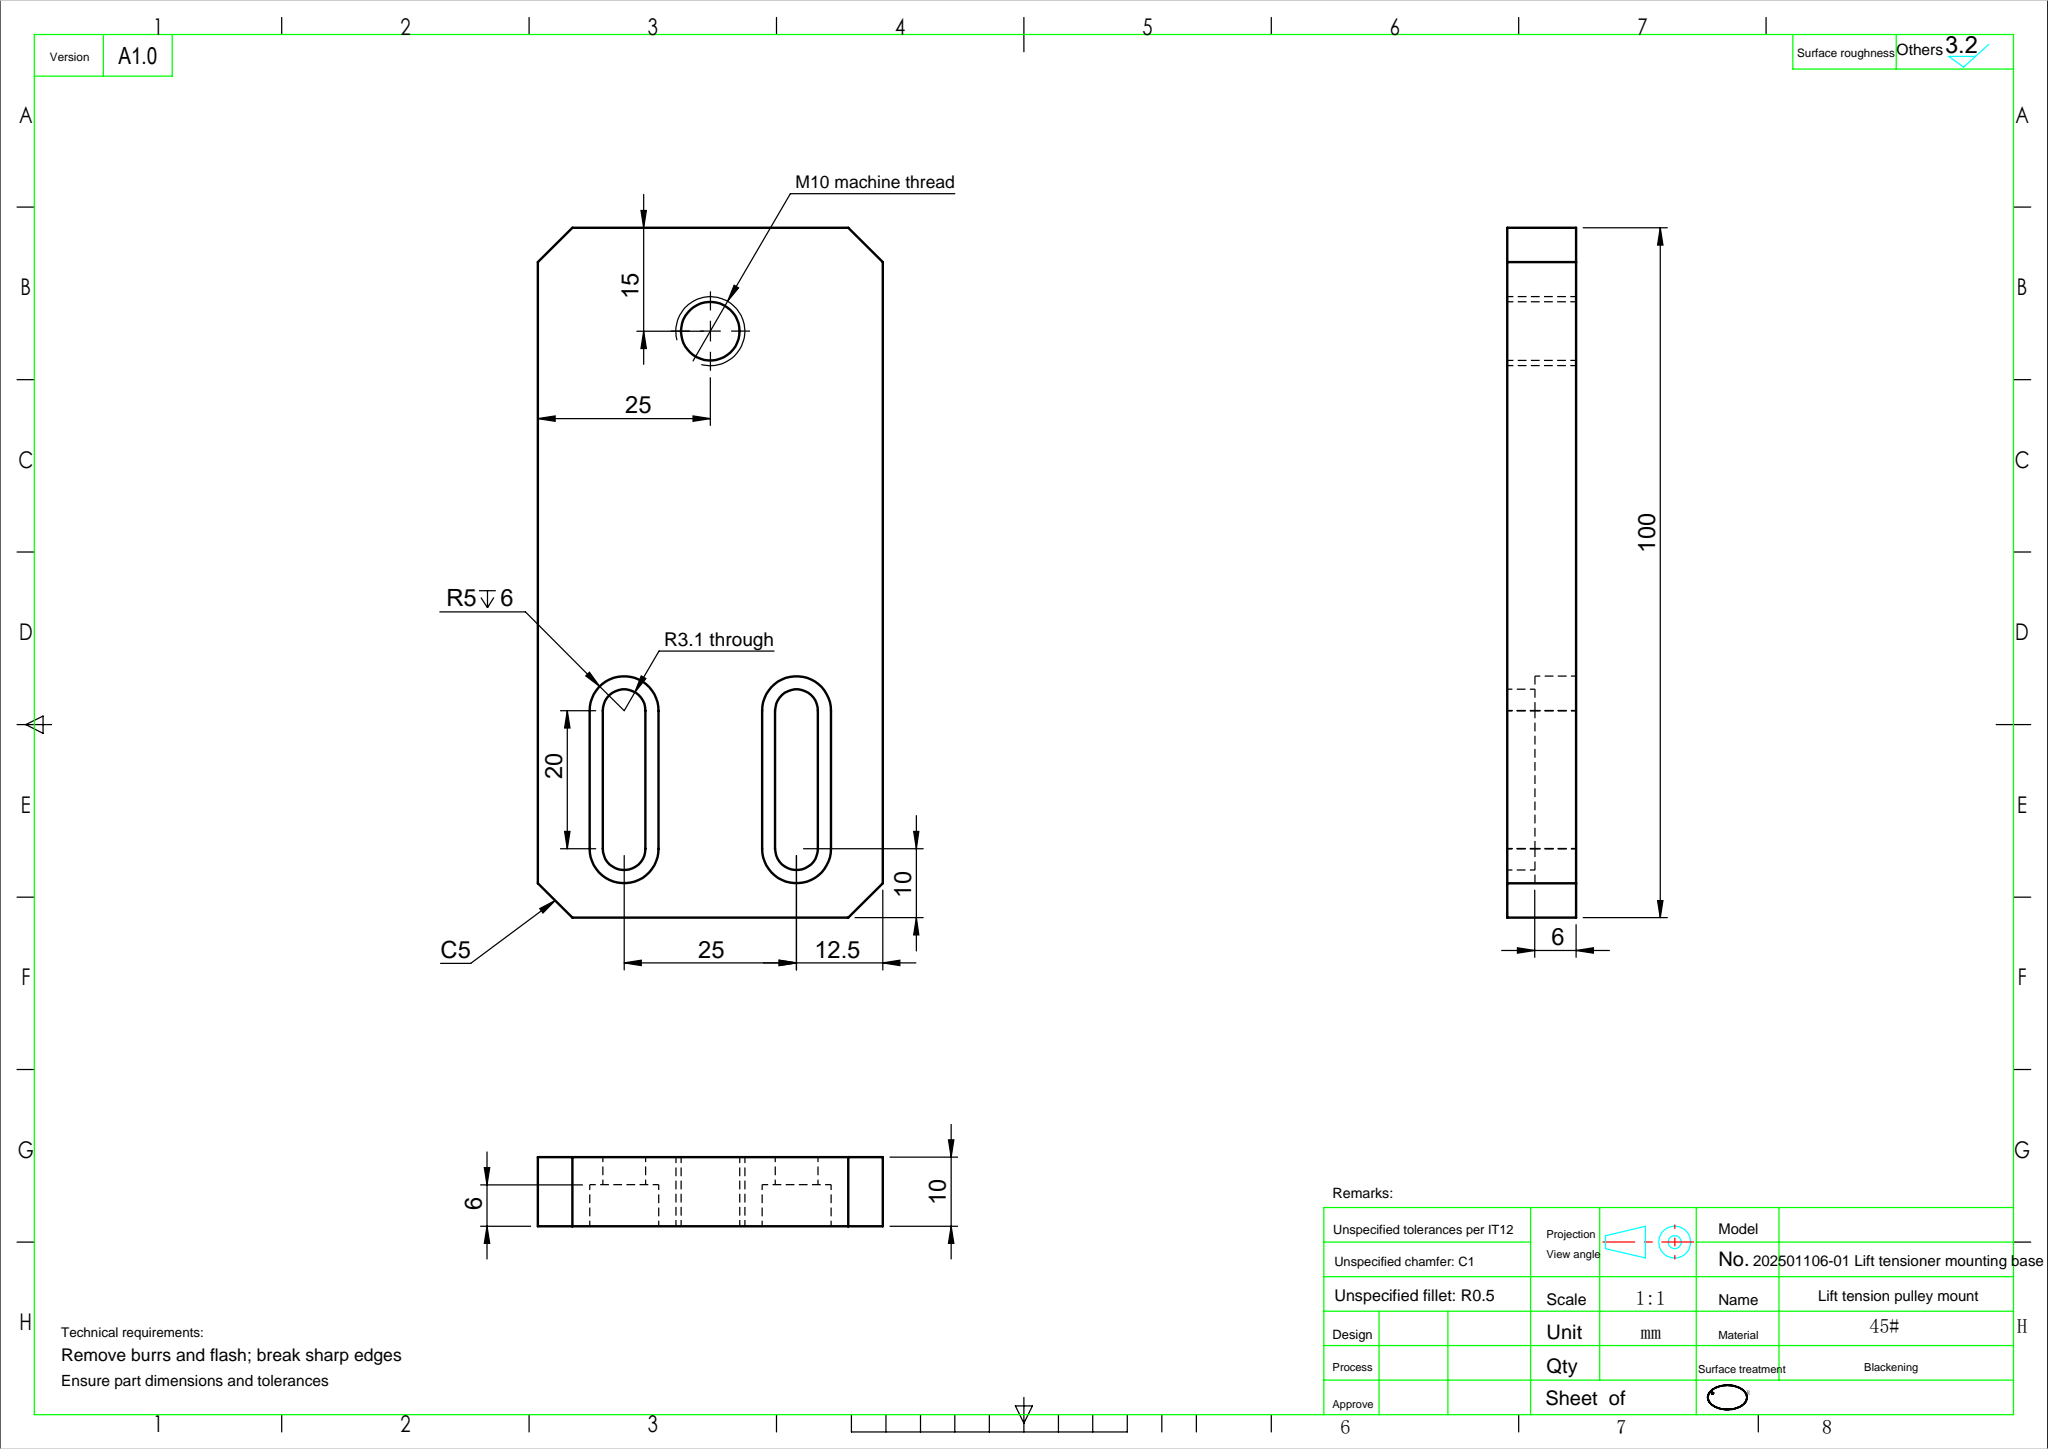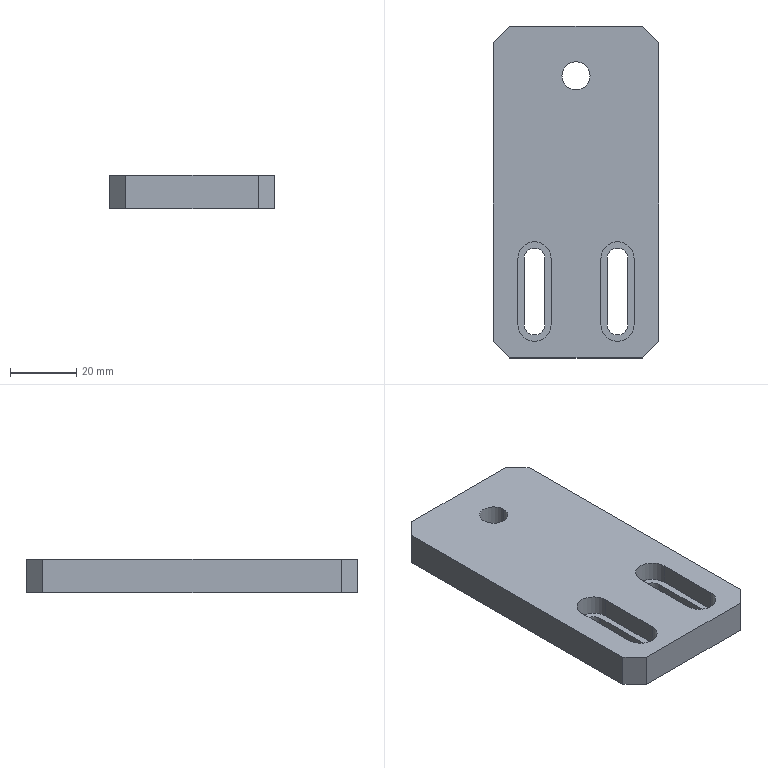Part | SolidWorks | features ICE 3, Chamfer 1, Extrusion 1 | 1 solid | 30 faces | box 50 x 100 x 10 mm | volume 44357 mm3 | plane 20 | cylinder 10 | commonest cylinder face diameters 6.2 x4 10 x4 8.5 x2
STEP:
#1=CARTESIAN_POINT('',(-4.25,35.,0.));
#2=VERTEX_POINT('',#1);
#3=CARTESIAN_POINT('',(4.25,35.,0.));
#4=VERTEX_POINT('',#3);
#5=CARTESIAN_POINT('',(0.,35.,0.));
#6=DIRECTION('',(0.,0.,1.));
#7=DIRECTION('',(1.,0.,0.));
#8=AXIS2_PLACEMENT_3D('',#5,#6,#7);
#9=CIRCLE('',#8,4.25);
#10=EDGE_CURVE('',#2,#4,#9,.T.);
#11=ORIENTED_EDGE('',*,*,#10,.F.);
#12=CARTESIAN_POINT('',(-4.25,35.,10.));
#13=VERTEX_POINT('',#12);
#14=CARTESIAN_POINT('',(-4.25,35.,0.));
#15=DIRECTION('',(0.,0.,1.));
#16=VECTOR('',#15,1000.);
#17=LINE('',#14,#16);
#18=EDGE_CURVE('',#2,#13,#17,.T.);
#19=ORIENTED_EDGE('',*,*,#18,.T.);
#20=CARTESIAN_POINT('',(4.25,35.,10.));
#21=VERTEX_POINT('',#20);
#22=CARTESIAN_POINT('',(0.,35.,10.));
#23=DIRECTION('',(0.,0.,1.));
#24=DIRECTION('',(1.,0.,0.));
#25=AXIS2_PLACEMENT_3D('',#22,#23,#24);
#26=CIRCLE('',#25,4.25);
#27=EDGE_CURVE('',#13,#21,#26,.T.);
#28=ORIENTED_EDGE('',*,*,#27,.T.);
#29=CARTESIAN_POINT('',(4.25,35.,0.));
#30=DIRECTION('',(0.,0.,1.));
#31=VECTOR('',#30,1000.);
#32=LINE('',#29,#31);
#33=EDGE_CURVE('',#4,#21,#32,.T.);
#34=ORIENTED_EDGE('',*,*,#33,.F.);
#35=EDGE_LOOP('',(#11,#19,#28,#34));
#36=FACE_OUTER_BOUND('',#35,.T.);
#37=CARTESIAN_POINT('',(0.,35.,0.));
#38=DIRECTION('',(0.,0.,1.));
#39=DIRECTION('',(1.,0.,0.));
#40=AXIS2_PLACEMENT_3D('',#37,#38,#39);
#41=CYLINDRICAL_SURFACE('',#40,4.25);
#42=ADVANCED_FACE('',(#36),#41,.F.);
#43=CARTESIAN_POINT('',(15.6,-40.,4.));
#44=VERTEX_POINT('',#43);
#45=CARTESIAN_POINT('',(9.4,-40.,4.));
#46=VERTEX_POINT('',#45);
#47=CARTESIAN_POINT('',(12.5,-40.,4.));
#48=DIRECTION('',(0.,0.,-1.));
#49=DIRECTION('',(1.,0.,0.));
#50=AXIS2_PLACEMENT_3D('',#47,#48,#49);
#51=CIRCLE('',#50,3.1);
#52=EDGE_CURVE('',#44,#46,#51,.T.);
#53=ORIENTED_EDGE('',*,*,#52,.F.);
#54=CARTESIAN_POINT('',(15.6,-40.,0.));
#55=VERTEX_POINT('',#54);
#56=CARTESIAN_POINT('',(15.6,-40.,0.));
#57=DIRECTION('',(0.,0.,1.));
#58=VECTOR('',#57,1000.);
#59=LINE('',#56,#58);
#60=EDGE_CURVE('',#55,#44,#59,.T.);
#61=ORIENTED_EDGE('',*,*,#60,.F.);
#62=CARTESIAN_POINT('',(9.4,-40.,0.));
#63=VERTEX_POINT('',#62);
#64=CARTESIAN_POINT('',(12.5,-40.,0.));
#65=DIRECTION('',(0.,0.,1.));
#66=DIRECTION('',(1.,0.,0.));
#67=AXIS2_PLACEMENT_3D('',#64,#65,#66);
#68=CIRCLE('',#67,3.1);
#69=EDGE_CURVE('',#63,#55,#68,.T.);
#70=ORIENTED_EDGE('',*,*,#69,.F.);
#71=CARTESIAN_POINT('',(9.4,-40.,0.));
#72=DIRECTION('',(0.,0.,1.));
#73=VECTOR('',#72,1000.);
#74=LINE('',#71,#73);
#75=EDGE_CURVE('',#63,#46,#74,.T.);
#76=ORIENTED_EDGE('',*,*,#75,.T.);
#77=EDGE_LOOP('',(#53,#61,#70,#76));
#78=FACE_OUTER_BOUND('',#77,.T.);
#79=CARTESIAN_POINT('',(12.5,-40.,0.));
#80=DIRECTION('',(0.,0.,1.));
#81=DIRECTION('',(1.,0.,0.));
#82=AXIS2_PLACEMENT_3D('',#79,#80,#81);
#83=CYLINDRICAL_SURFACE('',#82,3.1);
#84=ADVANCED_FACE('',(#78),#83,.F.);
#85=CARTESIAN_POINT('',(9.4,-20.,4.));
#86=VERTEX_POINT('',#85);
#87=CARTESIAN_POINT('',(9.4,-40.,4.));
#88=DIRECTION('',(0.,1.,0.));
#89=VECTOR('',#88,1000.);
#90=LINE('',#87,#89);
#91=EDGE_CURVE('',#46,#86,#90,.T.);
#92=ORIENTED_EDGE('',*,*,#91,.F.);
#93=ORIENTED_EDGE('',*,*,#75,.F.);
#94=CARTESIAN_POINT('',(9.4,-20.,0.));
#95=VERTEX_POINT('',#94);
#96=CARTESIAN_POINT('',(9.4,-40.,0.));
#97=DIRECTION('',(0.,-1.,0.));
#98=VECTOR('',#97,1000.);
#99=LINE('',#96,#98);
#100=EDGE_CURVE('',#95,#63,#99,.T.);
#101=ORIENTED_EDGE('',*,*,#100,.F.);
#102=CARTESIAN_POINT('',(9.4,-20.,0.));
#103=DIRECTION('',(0.,0.,1.));
#104=VECTOR('',#103,1000.);
#105=LINE('',#102,#104);
#106=EDGE_CURVE('',#95,#86,#105,.T.);
#107=ORIENTED_EDGE('',*,*,#106,.T.);
#108=EDGE_LOOP('',(#92,#93,#101,#107));
#109=FACE_OUTER_BOUND('',#108,.T.);
#110=CARTESIAN_POINT('',(9.4,-40.,0.));
#111=DIRECTION('',(-1.,0.,0.));
#112=DIRECTION('',(0.,0.,1.));
#113=AXIS2_PLACEMENT_3D('',#110,#111,#112);
#114=PLANE('',#113);
#115=ADVANCED_FACE('',(#109),#114,.F.);
#116=CARTESIAN_POINT('',(15.6,-20.,4.));
#117=VERTEX_POINT('',#116);
#118=CARTESIAN_POINT('',(12.5,-20.,4.));
#119=DIRECTION('',(0.,0.,-1.));
#120=DIRECTION('',(1.,0.,0.));
#121=AXIS2_PLACEMENT_3D('',#118,#119,#120);
#122=CIRCLE('',#121,3.1);
#123=EDGE_CURVE('',#86,#117,#122,.T.);
#124=ORIENTED_EDGE('',*,*,#123,.F.);
#125=ORIENTED_EDGE('',*,*,#106,.F.);
#126=CARTESIAN_POINT('',(15.6,-20.,0.));
#127=VERTEX_POINT('',#126);
#128=CARTESIAN_POINT('',(12.5,-20.,0.));
#129=DIRECTION('',(0.,0.,1.));
#130=DIRECTION('',(1.,0.,0.));
#131=AXIS2_PLACEMENT_3D('',#128,#129,#130);
#132=CIRCLE('',#131,3.1);
#133=EDGE_CURVE('',#127,#95,#132,.T.);
#134=ORIENTED_EDGE('',*,*,#133,.F.);
#135=CARTESIAN_POINT('',(15.6,-20.,0.));
#136=DIRECTION('',(0.,0.,1.));
#137=VECTOR('',#136,1000.);
#138=LINE('',#135,#137);
#139=EDGE_CURVE('',#127,#117,#138,.T.);
#140=ORIENTED_EDGE('',*,*,#139,.T.);
#141=EDGE_LOOP('',(#124,#125,#134,#140));
#142=FACE_OUTER_BOUND('',#141,.T.);
#143=CARTESIAN_POINT('',(12.5,-20.,0.));
#144=DIRECTION('',(0.,0.,1.));
#145=DIRECTION('',(1.,0.,0.));
#146=AXIS2_PLACEMENT_3D('',#143,#144,#145);
#147=CYLINDRICAL_SURFACE('',#146,3.1);
#148=ADVANCED_FACE('',(#142),#147,.F.);
#149=CARTESIAN_POINT('',(15.6,-40.,4.));
#150=DIRECTION('',(0.,-1.,0.));
#151=VECTOR('',#150,1000.);
#152=LINE('',#149,#151);
#153=EDGE_CURVE('',#117,#44,#152,.T.);
#154=ORIENTED_EDGE('',*,*,#153,.F.);
#155=ORIENTED_EDGE('',*,*,#139,.F.);
#156=CARTESIAN_POINT('',(15.6,-40.,0.));
#157=DIRECTION('',(0.,1.,0.));
#158=VECTOR('',#157,1000.);
#159=LINE('',#156,#158);
#160=EDGE_CURVE('',#55,#127,#159,.T.);
#161=ORIENTED_EDGE('',*,*,#160,.F.);
#162=ORIENTED_EDGE('',*,*,#60,.T.);
#163=EDGE_LOOP('',(#154,#155,#161,#162));
#164=FACE_OUTER_BOUND('',#163,.T.);
#165=CARTESIAN_POINT('',(15.6,-40.,0.));
#166=DIRECTION('',(1.,0.,0.));
#167=DIRECTION('',(0.,0.,-1.));
#168=AXIS2_PLACEMENT_3D('',#165,#166,#167);
#169=PLANE('',#168);
#170=ADVANCED_FACE('',(#164),#169,.F.);
#171=CARTESIAN_POINT('',(-15.6,-20.,4.));
#172=VERTEX_POINT('',#171);
#173=CARTESIAN_POINT('',(-9.4,-20.,4.));
#174=VERTEX_POINT('',#173);
#175=CARTESIAN_POINT('',(-12.5,-20.,4.));
#176=DIRECTION('',(0.,0.,-1.));
#177=DIRECTION('',(1.,0.,0.));
#178=AXIS2_PLACEMENT_3D('',#175,#176,#177);
#179=CIRCLE('',#178,3.1);
#180=EDGE_CURVE('',#172,#174,#179,.T.);
#181=ORIENTED_EDGE('',*,*,#180,.F.);
#182=CARTESIAN_POINT('',(-15.6,-20.,0.));
#183=VERTEX_POINT('',#182);
#184=CARTESIAN_POINT('',(-15.6,-20.,0.));
#185=DIRECTION('',(0.,0.,1.));
#186=VECTOR('',#185,1000.);
#187=LINE('',#184,#186);
#188=EDGE_CURVE('',#183,#172,#187,.T.);
#189=ORIENTED_EDGE('',*,*,#188,.F.);
#190=CARTESIAN_POINT('',(-9.4,-20.,0.));
#191=VERTEX_POINT('',#190);
#192=CARTESIAN_POINT('',(-12.5,-20.,0.));
#193=DIRECTION('',(0.,0.,1.));
#194=DIRECTION('',(1.,0.,0.));
#195=AXIS2_PLACEMENT_3D('',#192,#193,#194);
#196=CIRCLE('',#195,3.1);
#197=EDGE_CURVE('',#191,#183,#196,.T.);
#198=ORIENTED_EDGE('',*,*,#197,.F.);
#199=CARTESIAN_POINT('',(-9.4,-20.,0.));
#200=DIRECTION('',(0.,0.,1.));
#201=VECTOR('',#200,1000.);
#202=LINE('',#199,#201);
#203=EDGE_CURVE('',#191,#174,#202,.T.);
#204=ORIENTED_EDGE('',*,*,#203,.T.);
#205=EDGE_LOOP('',(#181,#189,#198,#204));
#206=FACE_OUTER_BOUND('',#205,.T.);
#207=CARTESIAN_POINT('',(-12.5,-20.,0.));
#208=DIRECTION('',(0.,0.,1.));
#209=DIRECTION('',(1.,0.,0.));
#210=AXIS2_PLACEMENT_3D('',#207,#208,#209);
#211=CYLINDRICAL_SURFACE('',#210,3.1);
#212=ADVANCED_FACE('',(#206),#211,.F.);
#213=CARTESIAN_POINT('',(-9.4,-40.,4.));
#214=VERTEX_POINT('',#213);
#215=CARTESIAN_POINT('',(-9.4,-20.,4.));
#216=DIRECTION('',(0.,-1.,0.));
#217=VECTOR('',#216,1000.);
#218=LINE('',#215,#217);
#219=EDGE_CURVE('',#174,#214,#218,.T.);
#220=ORIENTED_EDGE('',*,*,#219,.F.);
#221=ORIENTED_EDGE('',*,*,#203,.F.);
#222=CARTESIAN_POINT('',(-9.4,-40.,0.));
#223=VERTEX_POINT('',#222);
#224=CARTESIAN_POINT('',(-9.4,-20.,0.));
#225=DIRECTION('',(0.,1.,0.));
#226=VECTOR('',#225,1000.);
#227=LINE('',#224,#226);
#228=EDGE_CURVE('',#223,#191,#227,.T.);
#229=ORIENTED_EDGE('',*,*,#228,.F.);
#230=CARTESIAN_POINT('',(-9.4,-40.,0.));
#231=DIRECTION('',(0.,0.,1.));
#232=VECTOR('',#231,1000.);
#233=LINE('',#230,#232);
#234=EDGE_CURVE('',#223,#214,#233,.T.);
#235=ORIENTED_EDGE('',*,*,#234,.T.);
#236=EDGE_LOOP('',(#220,#221,#229,#235));
#237=FACE_OUTER_BOUND('',#236,.T.);
#238=CARTESIAN_POINT('',(-9.4,-20.,0.));
#239=DIRECTION('',(1.,0.,0.));
#240=DIRECTION('',(0.,1.,0.));
#241=AXIS2_PLACEMENT_3D('',#238,#239,#240);
#242=PLANE('',#241);
#243=ADVANCED_FACE('',(#237),#242,.F.);
#244=CARTESIAN_POINT('',(-15.6,-40.,4.));
#245=VERTEX_POINT('',#244);
#246=CARTESIAN_POINT('',(-12.5,-40.,4.));
#247=DIRECTION('',(0.,0.,-1.));
#248=DIRECTION('',(1.,0.,0.));
#249=AXIS2_PLACEMENT_3D('',#246,#247,#248);
#250=CIRCLE('',#249,3.1);
#251=EDGE_CURVE('',#214,#245,#250,.T.);
#252=ORIENTED_EDGE('',*,*,#251,.F.);
#253=ORIENTED_EDGE('',*,*,#234,.F.);
#254=CARTESIAN_POINT('',(-15.6,-40.,0.));
#255=VERTEX_POINT('',#254);
#256=CARTESIAN_POINT('',(-12.5,-40.,0.));
#257=DIRECTION('',(0.,0.,1.));
#258=DIRECTION('',(1.,0.,0.));
#259=AXIS2_PLACEMENT_3D('',#256,#257,#258);
#260=CIRCLE('',#259,3.1);
#261=EDGE_CURVE('',#255,#223,#260,.T.);
#262=ORIENTED_EDGE('',*,*,#261,.F.);
#263=CARTESIAN_POINT('',(-15.6,-40.,0.));
#264=DIRECTION('',(0.,0.,1.));
#265=VECTOR('',#264,1000.);
#266=LINE('',#263,#265);
#267=EDGE_CURVE('',#255,#245,#266,.T.);
#268=ORIENTED_EDGE('',*,*,#267,.T.);
#269=EDGE_LOOP('',(#252,#253,#262,#268));
#270=FACE_OUTER_BOUND('',#269,.T.);
#271=CARTESIAN_POINT('',(-12.5,-40.,0.));
#272=DIRECTION('',(0.,0.,1.));
#273=DIRECTION('',(1.,0.,0.));
#274=AXIS2_PLACEMENT_3D('',#271,#272,#273);
#275=CYLINDRICAL_SURFACE('',#274,3.1);
#276=ADVANCED_FACE('',(#270),#275,.F.);
#277=CARTESIAN_POINT('',(-15.6,-20.,4.));
#278=DIRECTION('',(0.,1.,0.));
#279=VECTOR('',#278,1000.);
#280=LINE('',#277,#279);
#281=EDGE_CURVE('',#245,#172,#280,.T.);
#282=ORIENTED_EDGE('',*,*,#281,.F.);
#283=ORIENTED_EDGE('',*,*,#267,.F.);
#284=CARTESIAN_POINT('',(-15.6,-20.,0.));
#285=DIRECTION('',(0.,-1.,0.));
#286=VECTOR('',#285,1000.);
#287=LINE('',#284,#286);
#288=EDGE_CURVE('',#183,#255,#287,.T.);
#289=ORIENTED_EDGE('',*,*,#288,.F.);
#290=ORIENTED_EDGE('',*,*,#188,.T.);
#291=EDGE_LOOP('',(#282,#283,#289,#290));
#292=FACE_OUTER_BOUND('',#291,.T.);
#293=CARTESIAN_POINT('',(-15.6,-20.,0.));
#294=DIRECTION('',(-1.,0.,0.));
#295=DIRECTION('',(0.,0.,1.));
#296=AXIS2_PLACEMENT_3D('',#293,#294,#295);
#297=PLANE('',#296);
#298=ADVANCED_FACE('',(#292),#297,.F.);
#299=CARTESIAN_POINT('',(25.,-45.,0.));
#300=VERTEX_POINT('',#299);
#301=CARTESIAN_POINT('',(25.,45.,0.));
#302=VERTEX_POINT('',#301);
#303=CARTESIAN_POINT('',(25.,50.,0.));
#304=DIRECTION('',(0.,1.,0.));
#305=VECTOR('',#304,1000.);
#306=LINE('',#303,#305);
#307=EDGE_CURVE('',#300,#302,#306,.T.);
#308=ORIENTED_EDGE('',*,*,#307,.T.);
#309=CARTESIAN_POINT('',(25.,45.,10.));
#310=VERTEX_POINT('',#309);
#311=CARTESIAN_POINT('',(25.,45.,10.));
#312=DIRECTION('',(0.,0.,1.));
#313=VECTOR('',#312,1000.);
#314=LINE('',#311,#313);
#315=EDGE_CURVE('',#302,#310,#314,.T.);
#316=ORIENTED_EDGE('',*,*,#315,.T.);
#317=CARTESIAN_POINT('',(25.,-45.,10.));
#318=VERTEX_POINT('',#317);
#319=CARTESIAN_POINT('',(25.,50.,10.));
#320=DIRECTION('',(0.,1.,0.));
#321=VECTOR('',#320,1000.);
#322=LINE('',#319,#321);
#323=EDGE_CURVE('',#318,#310,#322,.T.);
#324=ORIENTED_EDGE('',*,*,#323,.F.);
#325=CARTESIAN_POINT('',(25.,-45.,10.));
#326=DIRECTION('',(0.,0.,-1.));
#327=VECTOR('',#326,1000.);
#328=LINE('',#325,#327);
#329=EDGE_CURVE('',#318,#300,#328,.T.);
#330=ORIENTED_EDGE('',*,*,#329,.T.);
#331=EDGE_LOOP('',(#308,#316,#324,#330));
#332=FACE_OUTER_BOUND('',#331,.T.);
#333=CARTESIAN_POINT('',(25.,50.,10.));
#334=DIRECTION('',(-1.,0.,0.));
#335=DIRECTION('',(0.,0.,1.));
#336=AXIS2_PLACEMENT_3D('',#333,#334,#335);
#337=PLANE('',#336);
#338=ADVANCED_FACE('',(#332),#337,.F.);
#339=CARTESIAN_POINT('',(20.,50.,10.));
#340=VERTEX_POINT('',#339);
#341=CARTESIAN_POINT('',(-20.,50.,10.));
#342=VERTEX_POINT('',#341);
#343=CARTESIAN_POINT('',(-25.,50.,10.));
#344=DIRECTION('',(-1.,0.,0.));
#345=VECTOR('',#344,1000.);
#346=LINE('',#343,#345);
#347=EDGE_CURVE('',#340,#342,#346,.T.);
#348=ORIENTED_EDGE('',*,*,#347,.F.);
#349=CARTESIAN_POINT('',(20.,50.,0.));
#350=VERTEX_POINT('',#349);
#351=CARTESIAN_POINT('',(20.,50.,10.));
#352=DIRECTION('',(0.,0.,-1.));
#353=VECTOR('',#352,1000.);
#354=LINE('',#351,#353);
#355=EDGE_CURVE('',#340,#350,#354,.T.);
#356=ORIENTED_EDGE('',*,*,#355,.T.);
#357=CARTESIAN_POINT('',(-20.,50.,0.));
#358=VERTEX_POINT('',#357);
#359=CARTESIAN_POINT('',(-25.,50.,0.));
#360=DIRECTION('',(-1.,0.,0.));
#361=VECTOR('',#360,1000.);
#362=LINE('',#359,#361);
#363=EDGE_CURVE('',#350,#358,#362,.T.);
#364=ORIENTED_EDGE('',*,*,#363,.T.);
#365=CARTESIAN_POINT('',(-20.,50.,10.));
#366=DIRECTION('',(0.,0.,1.));
#367=VECTOR('',#366,1000.);
#368=LINE('',#365,#367);
#369=EDGE_CURVE('',#358,#342,#368,.T.);
#370=ORIENTED_EDGE('',*,*,#369,.T.);
#371=EDGE_LOOP('',(#348,#356,#364,#370));
#372=FACE_OUTER_BOUND('',#371,.T.);
#373=CARTESIAN_POINT('',(-25.,50.,10.));
#374=DIRECTION('',(0.,-1.,0.));
#375=DIRECTION('',(0.,0.,-1.));
#376=AXIS2_PLACEMENT_3D('',#373,#374,#375);
#377=PLANE('',#376);
#378=ADVANCED_FACE('',(#372),#377,.F.);
#379=CARTESIAN_POINT('',(-25.,45.,10.));
#380=VERTEX_POINT('',#379);
#381=CARTESIAN_POINT('',(-25.,-45.,10.));
#382=VERTEX_POINT('',#381);
#383=CARTESIAN_POINT('',(-25.,50.,10.));
#384=DIRECTION('',(0.,-1.,0.));
#385=VECTOR('',#384,1000.);
#386=LINE('',#383,#385);
#387=EDGE_CURVE('',#380,#382,#386,.T.);
#388=ORIENTED_EDGE('',*,*,#387,.F.);
#389=CARTESIAN_POINT('',(-25.,45.,0.));
#390=VERTEX_POINT('',#389);
#391=CARTESIAN_POINT('',(-25.,45.,10.));
#392=DIRECTION('',(0.,0.,-1.));
#393=VECTOR('',#392,1000.);
#394=LINE('',#391,#393);
#395=EDGE_CURVE('',#380,#390,#394,.T.);
#396=ORIENTED_EDGE('',*,*,#395,.T.);
#397=CARTESIAN_POINT('',(-25.,-45.,0.));
#398=VERTEX_POINT('',#397);
#399=CARTESIAN_POINT('',(-25.,50.,0.));
#400=DIRECTION('',(0.,-1.,0.));
#401=VECTOR('',#400,1000.);
#402=LINE('',#399,#401);
#403=EDGE_CURVE('',#390,#398,#402,.T.);
#404=ORIENTED_EDGE('',*,*,#403,.T.);
#405=CARTESIAN_POINT('',(-25.,-45.,10.));
#406=DIRECTION('',(0.,0.,1.));
#407=VECTOR('',#406,1000.);
#408=LINE('',#405,#407);
#409=EDGE_CURVE('',#398,#382,#408,.T.);
#410=ORIENTED_EDGE('',*,*,#409,.T.);
#411=EDGE_LOOP('',(#388,#396,#404,#410));
#412=FACE_OUTER_BOUND('',#411,.T.);
#413=CARTESIAN_POINT('',(-25.,50.,10.));
#414=DIRECTION('',(1.,0.,0.));
#415=DIRECTION('',(0.,0.,-1.));
#416=AXIS2_PLACEMENT_3D('',#413,#414,#415);
#417=PLANE('',#416);
#418=ADVANCED_FACE('',(#412),#417,.F.);
#419=CARTESIAN_POINT('',(-20.,-50.,0.));
#420=VERTEX_POINT('',#419);
#421=CARTESIAN_POINT('',(20.,-50.,0.));
#422=VERTEX_POINT('',#421);
#423=CARTESIAN_POINT('',(-25.,-50.,0.));
#424=DIRECTION('',(1.,0.,0.));
#425=VECTOR('',#424,1000.);
#426=LINE('',#423,#425);
#427=EDGE_CURVE('',#420,#422,#426,.T.);
#428=ORIENTED_EDGE('',*,*,#427,.T.);
#429=CARTESIAN_POINT('',(20.,-50.,10.));
#430=VERTEX_POINT('',#429);
#431=CARTESIAN_POINT('',(20.,-50.,10.));
#432=DIRECTION('',(0.,0.,1.));
#433=VECTOR('',#432,1000.);
#434=LINE('',#431,#433);
#435=EDGE_CURVE('',#422,#430,#434,.T.);
#436=ORIENTED_EDGE('',*,*,#435,.T.);
#437=CARTESIAN_POINT('',(-20.,-50.,10.));
#438=VERTEX_POINT('',#437);
#439=CARTESIAN_POINT('',(-25.,-50.,10.));
#440=DIRECTION('',(1.,0.,0.));
#441=VECTOR('',#440,1000.);
#442=LINE('',#439,#441);
#443=EDGE_CURVE('',#438,#430,#442,.T.);
#444=ORIENTED_EDGE('',*,*,#443,.F.);
#445=CARTESIAN_POINT('',(-20.,-50.,10.));
#446=DIRECTION('',(0.,0.,-1.));
#447=VECTOR('',#446,1000.);
#448=LINE('',#445,#447);
#449=EDGE_CURVE('',#438,#420,#448,.T.);
#450=ORIENTED_EDGE('',*,*,#449,.T.);
#451=EDGE_LOOP('',(#428,#436,#444,#450));
#452=FACE_OUTER_BOUND('',#451,.T.);
#453=CARTESIAN_POINT('',(-25.,-50.,10.));
#454=DIRECTION('',(0.,1.,0.));
#455=DIRECTION('',(0.,0.,1.));
#456=AXIS2_PLACEMENT_3D('',#453,#454,#455);
#457=PLANE('',#456);
#458=ADVANCED_FACE('',(#452),#457,.F.);
#459=CARTESIAN_POINT('',(0.,35.,10.));
#460=DIRECTION('',(0.,0.,1.));
#461=DIRECTION('',(1.,0.,0.));
#462=AXIS2_PLACEMENT_3D('',#459,#460,#461);
#463=CIRCLE('',#462,4.25);
#464=EDGE_CURVE('',#21,#13,#463,.T.);
#465=ORIENTED_EDGE('',*,*,#464,.F.);
#466=ORIENTED_EDGE('',*,*,#27,.F.);
#467=EDGE_LOOP('',(#465,#466));
#468=FACE_BOUND('',#467,.T.);
#469=CARTESIAN_POINT('',(-7.5,-20.,10.));
#470=VERTEX_POINT('',#469);
#471=CARTESIAN_POINT('',(-17.5,-20.,10.));
#472=VERTEX_POINT('',#471);
#473=CARTESIAN_POINT('',(-12.5,-20.,10.));
#474=DIRECTION('',(0.,0.,1.));
#475=DIRECTION('',(1.,0.,0.));
#476=AXIS2_PLACEMENT_3D('',#473,#474,#475);
#477=CIRCLE('',#476,5.);
#478=EDGE_CURVE('',#470,#472,#477,.T.);
#479=ORIENTED_EDGE('',*,*,#478,.F.);
#480=CARTESIAN_POINT('',(-7.5,-40.,10.));
#481=VERTEX_POINT('',#480);
#482=CARTESIAN_POINT('',(-7.5,-20.,10.));
#483=DIRECTION('',(0.,1.,0.));
#484=VECTOR('',#483,1000.);
#485=LINE('',#482,#484);
#486=EDGE_CURVE('',#481,#470,#485,.T.);
#487=ORIENTED_EDGE('',*,*,#486,.F.);
#488=CARTESIAN_POINT('',(-17.5,-40.,10.));
#489=VERTEX_POINT('',#488);
#490=CARTESIAN_POINT('',(-12.5,-40.,10.));
#491=DIRECTION('',(0.,0.,1.));
#492=DIRECTION('',(1.,0.,0.));
#493=AXIS2_PLACEMENT_3D('',#490,#491,#492);
#494=CIRCLE('',#493,5.);
#495=EDGE_CURVE('',#489,#481,#494,.T.);
#496=ORIENTED_EDGE('',*,*,#495,.F.);
#497=CARTESIAN_POINT('',(-17.5,-20.,10.));
#498=DIRECTION('',(0.,-1.,0.));
#499=VECTOR('',#498,1000.);
#500=LINE('',#497,#499);
#501=EDGE_CURVE('',#472,#489,#500,.T.);
#502=ORIENTED_EDGE('',*,*,#501,.F.);
#503=EDGE_LOOP('',(#479,#487,#496,#502));
#504=FACE_BOUND('',#503,.T.);
#505=CARTESIAN_POINT('',(17.5,-20.,10.));
#506=VERTEX_POINT('',#505);
#507=CARTESIAN_POINT('',(7.5,-20.,10.));
#508=VERTEX_POINT('',#507);
#509=CARTESIAN_POINT('',(12.5,-20.,10.));
#510=DIRECTION('',(0.,0.,1.));
#511=DIRECTION('',(1.,0.,0.));
#512=AXIS2_PLACEMENT_3D('',#509,#510,#511);
#513=CIRCLE('',#512,5.);
#514=EDGE_CURVE('',#506,#508,#513,.T.);
#515=ORIENTED_EDGE('',*,*,#514,.F.);
#516=CARTESIAN_POINT('',(17.5,-40.,10.));
#517=VERTEX_POINT('',#516);
#518=CARTESIAN_POINT('',(17.5,-20.,10.));
#519=DIRECTION('',(0.,1.,0.));
#520=VECTOR('',#519,1000.);
#521=LINE('',#518,#520);
#522=EDGE_CURVE('',#517,#506,#521,.T.);
#523=ORIENTED_EDGE('',*,*,#522,.F.);
#524=CARTESIAN_POINT('',(7.5,-40.,10.));
#525=VERTEX_POINT('',#524);
#526=CARTESIAN_POINT('',(12.5,-40.,10.));
#527=DIRECTION('',(0.,0.,1.));
#528=DIRECTION('',(1.,0.,0.));
#529=AXIS2_PLACEMENT_3D('',#526,#527,#528);
#530=CIRCLE('',#529,5.);
#531=EDGE_CURVE('',#525,#517,#530,.T.);
#532=ORIENTED_EDGE('',*,*,#531,.F.);
#533=CARTESIAN_POINT('',(7.5,-20.,10.));
#534=DIRECTION('',(0.,-1.,0.));
#535=VECTOR('',#534,1000.);
#536=LINE('',#533,#535);
#537=EDGE_CURVE('',#508,#525,#536,.T.);
#538=ORIENTED_EDGE('',*,*,#537,.F.);
#539=EDGE_LOOP('',(#515,#523,#532,#538));
#540=FACE_BOUND('',#539,.T.);
#541=ORIENTED_EDGE('',*,*,#323,.T.);
#542=CARTESIAN_POINT('',(35.,35.,10.));
#543=DIRECTION('',(-0.7071,0.7071,0.));
#544=VECTOR('',#543,1000.);
#545=LINE('',#542,#544);
#546=EDGE_CURVE('',#310,#340,#545,.T.);
#547=ORIENTED_EDGE('',*,*,#546,.T.);
#548=ORIENTED_EDGE('',*,*,#347,.T.);
#549=CARTESIAN_POINT('',(-35.,35.,10.));
#550=DIRECTION('',(-0.7071,-0.7071,0.));
#551=VECTOR('',#550,1000.);
#552=LINE('',#549,#551);
#553=EDGE_CURVE('',#342,#380,#552,.T.);
#554=ORIENTED_EDGE('',*,*,#553,.T.);
#555=ORIENTED_EDGE('',*,*,#387,.T.);
#556=CARTESIAN_POINT('',(-35.,-35.,10.));
#557=DIRECTION('',(0.7071,-0.7071,0.));
#558=VECTOR('',#557,1000.);
#559=LINE('',#556,#558);
#560=EDGE_CURVE('',#382,#438,#559,.T.);
#561=ORIENTED_EDGE('',*,*,#560,.T.);
#562=ORIENTED_EDGE('',*,*,#443,.T.);
#563=CARTESIAN_POINT('',(35.,-35.,10.));
#564=DIRECTION('',(0.7071,0.7071,0.));
#565=VECTOR('',#564,1000.);
#566=LINE('',#563,#565);
#567=EDGE_CURVE('',#430,#318,#566,.T.);
#568=ORIENTED_EDGE('',*,*,#567,.T.);
#569=EDGE_LOOP('',(#541,#547,#548,#554,#555,#561,#562,#568));
#570=FACE_OUTER_BOUND('',#569,.T.);
#571=CARTESIAN_POINT('',(0.,0.,10.));
#572=DIRECTION('',(0.,0.,1.));
#573=DIRECTION('',(1.,0.,0.));
#574=AXIS2_PLACEMENT_3D('',#571,#572,#573);
#575=PLANE('',#574);
#576=ADVANCED_FACE('',(#468,#504,#540,#570),#575,.T.);
#577=CARTESIAN_POINT('',(0.,35.,0.));
#578=DIRECTION('',(0.,0.,1.));
#579=DIRECTION('',(1.,0.,0.));
#580=AXIS2_PLACEMENT_3D('',#577,#578,#579);
#581=CIRCLE('',#580,4.25);
#582=EDGE_CURVE('',#4,#2,#581,.T.);
#583=ORIENTED_EDGE('',*,*,#582,.T.);
#584=ORIENTED_EDGE('',*,*,#10,.T.);
#585=EDGE_LOOP('',(#583,#584));
#586=FACE_BOUND('',#585,.T.);
#587=ORIENTED_EDGE('',*,*,#228,.T.);
#588=ORIENTED_EDGE('',*,*,#197,.T.);
#589=ORIENTED_EDGE('',*,*,#288,.T.);
#590=ORIENTED_EDGE('',*,*,#261,.T.);
#591=EDGE_LOOP('',(#587,#588,#589,#590));
#592=FACE_BOUND('',#591,.T.);
#593=ORIENTED_EDGE('',*,*,#100,.T.);
#594=ORIENTED_EDGE('',*,*,#69,.T.);
#595=ORIENTED_EDGE('',*,*,#160,.T.);
#596=ORIENTED_EDGE('',*,*,#133,.T.);
#597=EDGE_LOOP('',(#593,#594,#595,#596));
#598=FACE_BOUND('',#597,.T.);
#599=ORIENTED_EDGE('',*,*,#363,.F.);
#600=CARTESIAN_POINT('',(20.,50.,0.));
#601=DIRECTION('',(0.7071,-0.7071,0.));
#602=VECTOR('',#601,1000.);
#603=LINE('',#600,#602);
#604=EDGE_CURVE('',#350,#302,#603,.T.);
#605=ORIENTED_EDGE('',*,*,#604,.T.);
#606=ORIENTED_EDGE('',*,*,#307,.F.);
#607=CARTESIAN_POINT('',(25.,-45.,0.));
#608=DIRECTION('',(-0.7071,-0.7071,0.));
#609=VECTOR('',#608,1000.);
#610=LINE('',#607,#609);
#611=EDGE_CURVE('',#300,#422,#610,.T.);
#612=ORIENTED_EDGE('',*,*,#611,.T.);
#613=ORIENTED_EDGE('',*,*,#427,.F.);
#614=CARTESIAN_POINT('',(-20.,-50.,0.));
#615=DIRECTION('',(-0.7071,0.7071,0.));
#616=VECTOR('',#615,1000.);
#617=LINE('',#614,#616);
#618=EDGE_CURVE('',#420,#398,#617,.T.);
#619=ORIENTED_EDGE('',*,*,#618,.T.);
#620=ORIENTED_EDGE('',*,*,#403,.F.);
#621=CARTESIAN_POINT('',(-25.,45.,0.));
#622=DIRECTION('',(0.7071,0.7071,0.));
#623=VECTOR('',#622,1000.);
#624=LINE('',#621,#623);
#625=EDGE_CURVE('',#390,#358,#624,.T.);
#626=ORIENTED_EDGE('',*,*,#625,.T.);
#627=EDGE_LOOP('',(#599,#605,#606,#612,#613,#619,#620,#626));
#628=FACE_OUTER_BOUND('',#627,.T.);
#629=CARTESIAN_POINT('',(0.,0.,0.));
#630=DIRECTION('',(0.,0.,1.));
#631=DIRECTION('',(1.,0.,0.));
#632=AXIS2_PLACEMENT_3D('',#629,#630,#631);
#633=PLANE('',#632);
#634=ADVANCED_FACE('',(#586,#592,#598,#628),#633,.F.);
#635=CARTESIAN_POINT('',(-7.5,-20.,4.));
#636=VERTEX_POINT('',#635);
#637=CARTESIAN_POINT('',(-17.5,-20.,4.));
#638=VERTEX_POINT('',#637);
#639=CARTESIAN_POINT('',(-12.5,-20.,4.));
#640=DIRECTION('',(0.,0.,1.));
#641=DIRECTION('',(1.,0.,0.));
#642=AXIS2_PLACEMENT_3D('',#639,#640,#641);
#643=CIRCLE('',#642,5.);
#644=EDGE_CURVE('',#636,#638,#643,.T.);
#645=ORIENTED_EDGE('',*,*,#644,.T.);
#646=CARTESIAN_POINT('',(-17.5,-40.,4.));
#647=VERTEX_POINT('',#646);
#648=CARTESIAN_POINT('',(-17.5,-20.,4.));
#649=DIRECTION('',(0.,-1.,0.));
#650=VECTOR('',#649,1000.);
#651=LINE('',#648,#650);
#652=EDGE_CURVE('',#638,#647,#651,.T.);
#653=ORIENTED_EDGE('',*,*,#652,.T.);
#654=CARTESIAN_POINT('',(-7.5,-40.,4.));
#655=VERTEX_POINT('',#654);
#656=CARTESIAN_POINT('',(-12.5,-40.,4.));
#657=DIRECTION('',(0.,0.,1.));
#658=DIRECTION('',(1.,0.,0.));
#659=AXIS2_PLACEMENT_3D('',#656,#657,#658);
#660=CIRCLE('',#659,5.);
#661=EDGE_CURVE('',#647,#655,#660,.T.);
#662=ORIENTED_EDGE('',*,*,#661,.T.);
#663=CARTESIAN_POINT('',(-7.5,-20.,4.));
#664=DIRECTION('',(0.,1.,0.));
#665=VECTOR('',#664,1000.);
#666=LINE('',#663,#665);
#667=EDGE_CURVE('',#655,#636,#666,.T.);
#668=ORIENTED_EDGE('',*,*,#667,.T.);
#669=EDGE_LOOP('',(#645,#653,#662,#668));
#670=FACE_OUTER_BOUND('',#669,.T.);
#671=ORIENTED_EDGE('',*,*,#180,.T.);
#672=ORIENTED_EDGE('',*,*,#219,.T.);
#673=ORIENTED_EDGE('',*,*,#251,.T.);
#674=ORIENTED_EDGE('',*,*,#281,.T.);
#675=EDGE_LOOP('',(#671,#672,#673,#674));
#676=FACE_BOUND('',#675,.T.);
#677=CARTESIAN_POINT('',(-12.5,-20.,4.));
#678=DIRECTION('',(0.,0.,1.));
#679=DIRECTION('',(1.,0.,0.));
#680=AXIS2_PLACEMENT_3D('',#677,#678,#679);
#681=PLANE('',#680);
#682=ADVANCED_FACE('',(#670,#676),#681,.T.);
#683=ORIENTED_EDGE('',*,*,#478,.T.);
#684=CARTESIAN_POINT('',(-17.5,-20.,4.));
#685=DIRECTION('',(0.,0.,1.));
#686=VECTOR('',#685,1000.);
#687=LINE('',#684,#686);
#688=EDGE_CURVE('',#638,#472,#687,.T.);
#689=ORIENTED_EDGE('',*,*,#688,.F.);
#690=ORIENTED_EDGE('',*,*,#644,.F.);
#691=CARTESIAN_POINT('',(-7.5,-20.,4.));
#692=DIRECTION('',(0.,0.,1.));
#693=VECTOR('',#692,1000.);
#694=LINE('',#691,#693);
#695=EDGE_CURVE('',#636,#470,#694,.T.);
#696=ORIENTED_EDGE('',*,*,#695,.T.);
#697=EDGE_LOOP('',(#683,#689,#690,#696));
#698=FACE_OUTER_BOUND('',#697,.T.);
#699=CARTESIAN_POINT('',(-12.5,-20.,4.));
#700=DIRECTION('',(0.,0.,1.));
#701=DIRECTION('',(1.,0.,0.));
#702=AXIS2_PLACEMENT_3D('',#699,#700,#701);
#703=CYLINDRICAL_SURFACE('',#702,5.);
#704=ADVANCED_FACE('',(#698),#703,.F.);
#705=ORIENTED_EDGE('',*,*,#486,.T.);
#706=ORIENTED_EDGE('',*,*,#695,.F.);
#707=ORIENTED_EDGE('',*,*,#667,.F.);
#708=CARTESIAN_POINT('',(-7.5,-40.,4.));
#709=DIRECTION('',(0.,0.,1.));
#710=VECTOR('',#709,1000.);
#711=LINE('',#708,#710);
#712=EDGE_CURVE('',#655,#481,#711,.T.);
#713=ORIENTED_EDGE('',*,*,#712,.T.);
#714=EDGE_LOOP('',(#705,#706,#707,#713));
#715=FACE_OUTER_BOUND('',#714,.T.);
#716=CARTESIAN_POINT('',(-7.5,-20.,4.));
#717=DIRECTION('',(1.,0.,0.));
#718=DIRECTION('',(0.,1.,0.));
#719=AXIS2_PLACEMENT_3D('',#716,#717,#718);
#720=PLANE('',#719);
#721=ADVANCED_FACE('',(#715),#720,.F.);
#722=ORIENTED_EDGE('',*,*,#495,.T.);
#723=ORIENTED_EDGE('',*,*,#712,.F.);
#724=ORIENTED_EDGE('',*,*,#661,.F.);
#725=CARTESIAN_POINT('',(-17.5,-40.,4.));
#726=DIRECTION('',(0.,0.,1.));
#727=VECTOR('',#726,1000.);
#728=LINE('',#725,#727);
#729=EDGE_CURVE('',#647,#489,#728,.T.);
#730=ORIENTED_EDGE('',*,*,#729,.T.);
#731=EDGE_LOOP('',(#722,#723,#724,#730));
#732=FACE_OUTER_BOUND('',#731,.T.);
#733=CARTESIAN_POINT('',(-12.5,-40.,4.));
#734=DIRECTION('',(0.,0.,1.));
#735=DIRECTION('',(1.,0.,0.));
#736=AXIS2_PLACEMENT_3D('',#733,#734,#735);
#737=CYLINDRICAL_SURFACE('',#736,5.);
#738=ADVANCED_FACE('',(#732),#737,.F.);
#739=ORIENTED_EDGE('',*,*,#501,.T.);
#740=ORIENTED_EDGE('',*,*,#729,.F.);
#741=ORIENTED_EDGE('',*,*,#652,.F.);
#742=ORIENTED_EDGE('',*,*,#688,.T.);
#743=EDGE_LOOP('',(#739,#740,#741,#742));
#744=FACE_OUTER_BOUND('',#743,.T.);
#745=CARTESIAN_POINT('',(-17.5,-20.,4.));
#746=DIRECTION('',(-1.,0.,0.));
#747=DIRECTION('',(0.,0.,1.));
#748=AXIS2_PLACEMENT_3D('',#745,#746,#747);
#749=PLANE('',#748);
#750=ADVANCED_FACE('',(#744),#749,.F.);
#751=CARTESIAN_POINT('',(17.5,-20.,4.));
#752=VERTEX_POINT('',#751);
#753=CARTESIAN_POINT('',(7.5,-20.,4.));
#754=VERTEX_POINT('',#753);
#755=CARTESIAN_POINT('',(12.5,-20.,4.));
#756=DIRECTION('',(0.,0.,1.));
#757=DIRECTION('',(1.,0.,0.));
#758=AXIS2_PLACEMENT_3D('',#755,#756,#757);
#759=CIRCLE('',#758,5.);
#760=EDGE_CURVE('',#752,#754,#759,.T.);
#761=ORIENTED_EDGE('',*,*,#760,.T.);
#762=CARTESIAN_POINT('',(7.5,-40.,4.));
#763=VERTEX_POINT('',#762);
#764=CARTESIAN_POINT('',(7.5,-20.,4.));
#765=DIRECTION('',(0.,-1.,0.));
#766=VECTOR('',#765,1000.);
#767=LINE('',#764,#766);
#768=EDGE_CURVE('',#754,#763,#767,.T.);
#769=ORIENTED_EDGE('',*,*,#768,.T.);
#770=CARTESIAN_POINT('',(17.5,-40.,4.));
#771=VERTEX_POINT('',#770);
#772=CARTESIAN_POINT('',(12.5,-40.,4.));
#773=DIRECTION('',(0.,0.,1.));
#774=DIRECTION('',(1.,0.,0.));
#775=AXIS2_PLACEMENT_3D('',#772,#773,#774);
#776=CIRCLE('',#775,5.);
#777=EDGE_CURVE('',#763,#771,#776,.T.);
#778=ORIENTED_EDGE('',*,*,#777,.T.);
#779=CARTESIAN_POINT('',(17.5,-20.,4.));
#780=DIRECTION('',(0.,1.,0.));
#781=VECTOR('',#780,1000.);
#782=LINE('',#779,#781);
#783=EDGE_CURVE('',#771,#752,#782,.T.);
#784=ORIENTED_EDGE('',*,*,#783,.T.);
#785=EDGE_LOOP('',(#761,#769,#778,#784));
#786=FACE_OUTER_BOUND('',#785,.T.);
#787=ORIENTED_EDGE('',*,*,#52,.T.);
#788=ORIENTED_EDGE('',*,*,#91,.T.);
#789=ORIENTED_EDGE('',*,*,#123,.T.);
#790=ORIENTED_EDGE('',*,*,#153,.T.);
#791=EDGE_LOOP('',(#787,#788,#789,#790));
#792=FACE_BOUND('',#791,.T.);
#793=CARTESIAN_POINT('',(12.5,-20.,4.));
#794=DIRECTION('',(0.,0.,1.));
#795=DIRECTION('',(1.,0.,0.));
#796=AXIS2_PLACEMENT_3D('',#793,#794,#795);
#797=PLANE('',#796);
#798=ADVANCED_FACE('',(#786,#792),#797,.T.);
#799=ORIENTED_EDGE('',*,*,#514,.T.);
#800=CARTESIAN_POINT('',(7.5,-20.,4.));
#801=DIRECTION('',(0.,0.,1.));
#802=VECTOR('',#801,1000.);
#803=LINE('',#800,#802);
#804=EDGE_CURVE('',#754,#508,#803,.T.);
#805=ORIENTED_EDGE('',*,*,#804,.F.);
#806=ORIENTED_EDGE('',*,*,#760,.F.);
#807=CARTESIAN_POINT('',(17.5,-20.,4.));
#808=DIRECTION('',(0.,0.,1.));
#809=VECTOR('',#808,1000.);
#810=LINE('',#807,#809);
#811=EDGE_CURVE('',#752,#506,#810,.T.);
#812=ORIENTED_EDGE('',*,*,#811,.T.);
#813=EDGE_LOOP('',(#799,#805,#806,#812));
#814=FACE_OUTER_BOUND('',#813,.T.);
#815=CARTESIAN_POINT('',(12.5,-20.,4.));
#816=DIRECTION('',(0.,0.,1.));
#817=DIRECTION('',(1.,0.,0.));
#818=AXIS2_PLACEMENT_3D('',#815,#816,#817);
#819=CYLINDRICAL_SURFACE('',#818,5.);
#820=ADVANCED_FACE('',(#814),#819,.F.);
#821=ORIENTED_EDGE('',*,*,#522,.T.);
#822=ORIENTED_EDGE('',*,*,#811,.F.);
#823=ORIENTED_EDGE('',*,*,#783,.F.);
#824=CARTESIAN_POINT('',(17.5,-40.,4.));
#825=DIRECTION('',(0.,0.,1.));
#826=VECTOR('',#825,1000.);
#827=LINE('',#824,#826);
#828=EDGE_CURVE('',#771,#517,#827,.T.);
#829=ORIENTED_EDGE('',*,*,#828,.T.);
#830=EDGE_LOOP('',(#821,#822,#823,#829));
#831=FACE_OUTER_BOUND('',#830,.T.);
#832=CARTESIAN_POINT('',(17.5,-20.,4.));
#833=DIRECTION('',(1.,0.,0.));
#834=DIRECTION('',(0.,0.,-1.));
#835=AXIS2_PLACEMENT_3D('',#832,#833,#834);
#836=PLANE('',#835);
#837=ADVANCED_FACE('',(#831),#836,.F.);
#838=ORIENTED_EDGE('',*,*,#531,.T.);
#839=ORIENTED_EDGE('',*,*,#828,.F.);
#840=ORIENTED_EDGE('',*,*,#777,.F.);
#841=CARTESIAN_POINT('',(7.5,-40.,4.));
#842=DIRECTION('',(0.,0.,1.));
#843=VECTOR('',#842,1000.);
#844=LINE('',#841,#843);
#845=EDGE_CURVE('',#763,#525,#844,.T.);
#846=ORIENTED_EDGE('',*,*,#845,.T.);
#847=EDGE_LOOP('',(#838,#839,#840,#846));
#848=FACE_OUTER_BOUND('',#847,.T.);
#849=CARTESIAN_POINT('',(12.5,-40.,4.));
#850=DIRECTION('',(0.,0.,1.));
#851=DIRECTION('',(1.,0.,0.));
#852=AXIS2_PLACEMENT_3D('',#849,#850,#851);
#853=CYLINDRICAL_SURFACE('',#852,5.);
#854=ADVANCED_FACE('',(#848),#853,.F.);
#855=ORIENTED_EDGE('',*,*,#537,.T.);
#856=ORIENTED_EDGE('',*,*,#845,.F.);
#857=ORIENTED_EDGE('',*,*,#768,.F.);
#858=ORIENTED_EDGE('',*,*,#804,.T.);
#859=EDGE_LOOP('',(#855,#856,#857,#858));
#860=FACE_OUTER_BOUND('',#859,.T.);
#861=CARTESIAN_POINT('',(7.5,-20.,4.));
#862=DIRECTION('',(-1.,0.,0.));
#863=DIRECTION('',(0.,0.,1.));
#864=AXIS2_PLACEMENT_3D('',#861,#862,#863);
#865=PLANE('',#864);
#866=ADVANCED_FACE('',(#860),#865,.F.);
#867=ORIENTED_EDGE('',*,*,#546,.F.);
#868=ORIENTED_EDGE('',*,*,#315,.F.);
#869=ORIENTED_EDGE('',*,*,#604,.F.);
#870=ORIENTED_EDGE('',*,*,#355,.F.);
#871=EDGE_LOOP('',(#867,#868,#869,#870));
#872=FACE_OUTER_BOUND('',#871,.T.);
#873=CARTESIAN_POINT('',(20.,50.,10.));
#874=DIRECTION('',(-0.7071,-0.7071,0.));
#875=DIRECTION('',(0.,0.,-1.));
#876=AXIS2_PLACEMENT_3D('',#873,#874,#875);
#877=PLANE('',#876);
#878=ADVANCED_FACE('',(#872),#877,.F.);
#879=ORIENTED_EDGE('',*,*,#553,.F.);
#880=ORIENTED_EDGE('',*,*,#369,.F.);
#881=ORIENTED_EDGE('',*,*,#625,.F.);
#882=ORIENTED_EDGE('',*,*,#395,.F.);
#883=EDGE_LOOP('',(#879,#880,#881,#882));
#884=FACE_OUTER_BOUND('',#883,.T.);
#885=CARTESIAN_POINT('',(-25.,45.,10.));
#886=DIRECTION('',(0.7071,-0.7071,0.));
#887=DIRECTION('',(0.,0.,-1.));
#888=AXIS2_PLACEMENT_3D('',#885,#886,#887);
#889=PLANE('',#888);
#890=ADVANCED_FACE('',(#884),#889,.F.);
#891=ORIENTED_EDGE('',*,*,#567,.F.);
#892=ORIENTED_EDGE('',*,*,#435,.F.);
#893=ORIENTED_EDGE('',*,*,#611,.F.);
#894=ORIENTED_EDGE('',*,*,#329,.F.);
#895=EDGE_LOOP('',(#891,#892,#893,#894));
#896=FACE_OUTER_BOUND('',#895,.T.);
#897=CARTESIAN_POINT('',(25.,-45.,10.));
#898=DIRECTION('',(-0.7071,0.7071,0.));
#899=DIRECTION('',(0.,0.,-1.));
#900=AXIS2_PLACEMENT_3D('',#897,#898,#899);
#901=PLANE('',#900);
#902=ADVANCED_FACE('',(#896),#901,.F.);
#903=ORIENTED_EDGE('',*,*,#560,.F.);
#904=ORIENTED_EDGE('',*,*,#409,.F.);
#905=ORIENTED_EDGE('',*,*,#618,.F.);
#906=ORIENTED_EDGE('',*,*,#449,.F.);
#907=EDGE_LOOP('',(#903,#904,#905,#906));
#908=FACE_OUTER_BOUND('',#907,.T.);
#909=CARTESIAN_POINT('',(-20.,-50.,10.));
#910=DIRECTION('',(0.7071,0.7071,0.));
#911=DIRECTION('',(0.,0.,-1.));
#912=AXIS2_PLACEMENT_3D('',#909,#910,#911);
#913=PLANE('',#912);
#914=ADVANCED_FACE('',(#908),#913,.F.);
#915=ORIENTED_EDGE('',*,*,#18,.F.);
#916=ORIENTED_EDGE('',*,*,#582,.F.);
#917=ORIENTED_EDGE('',*,*,#33,.T.);
#918=ORIENTED_EDGE('',*,*,#464,.T.);
#919=EDGE_LOOP('',(#915,#916,#917,#918));
#920=FACE_OUTER_BOUND('',#919,.T.);
#921=CARTESIAN_POINT('',(0.,35.,0.));
#922=DIRECTION('',(0.,0.,1.));
#923=DIRECTION('',(1.,0.,0.));
#924=AXIS2_PLACEMENT_3D('',#921,#922,#923);
#925=CYLINDRICAL_SURFACE('',#924,4.25);
#926=ADVANCED_FACE('',(#920),#925,.F.);
#927=CLOSED_SHELL('',(#42,#84,#115,#148,#170,#212,#243,#276,#298,#338,#378,#418,#458,#576,#634,#682,#704,#721,#738,#750,#798,#820,#837,#854,#866,#878,#890,#902,#914,#926));
#928=MANIFOLD_SOLID_BREP('',#927);
#929=CARTESIAN_POINT('',(0.,0.,0.));
#930=DIRECTION('',(0.,0.,1.));
#931=DIRECTION('',(1.,0.,0.));
#932=AXIS2_PLACEMENT_3D('',#929,#930,#931);
#933=(LENGTH_UNIT()NAMED_UNIT(*)SI_UNIT(.MILLI.,.METRE.));
#934=UNCERTAINTY_MEASURE_WITH_UNIT(LENGTH_MEASURE(0.00001),#933,'','');
#935=(NAMED_UNIT(*)PLANE_ANGLE_UNIT()SI_UNIT($,.RADIAN.));
#936=(NAMED_UNIT(*)SI_UNIT($,.STERADIAN.)SOLID_ANGLE_UNIT());
#937=(GEOMETRIC_REPRESENTATION_CONTEXT(3)GLOBAL_UNCERTAINTY_ASSIGNED_CONTEXT((#934))GLOBAL_UNIT_ASSIGNED_CONTEXT((#933,#935,#936))REPRESENTATION_CONTEXT('',''));
#938=ADVANCED_BREP_SHAPE_REPRESENTATION('',(#928,#932),#937);